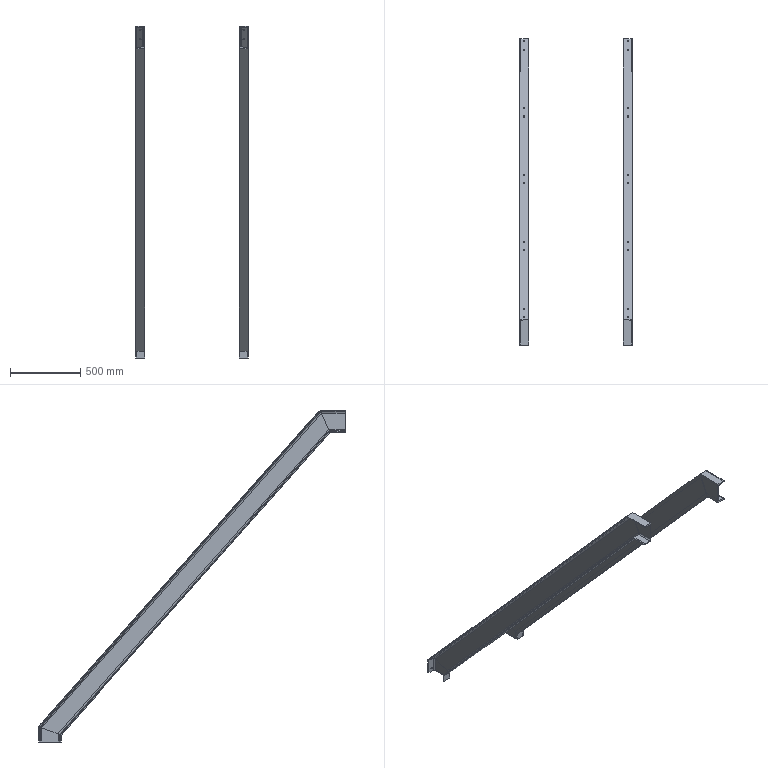Part | STEP file | Mirror_中转釜楼梯主体1_Default<As Machined> | 6 solids | 126 faces | box 800 x 2180 x 2360 mm | volume 13882190 mm3 | cylinder 66 | plane 60 | commonest cylinder face diameters 12 x40 10 x12 20 x12 13 x2